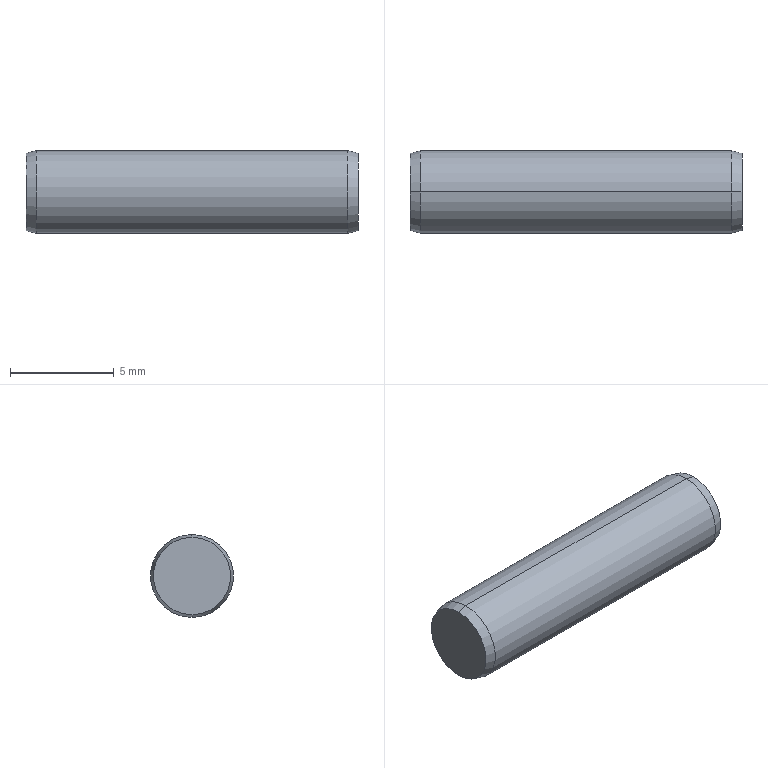Part | STEP file | GB/T 119 4×16 | 1 solid | 8 faces | box 16 x 4 x 4 mm | volume 200.239 mm3 | cone 4 | cylinder 2 | plane 2 | commonest cylinder face diameters 4 x2
STEP:
#1=CARTESIAN_POINT('',(14.,0.,2.));
#2=VERTEX_POINT('',#1);
#3=CARTESIAN_POINT('',(14.,0.,-2.));
#4=VERTEX_POINT('',#3);
#5=CARTESIAN_POINT('',(14.,0.,0.));
#6=DIRECTION('',(-1.,0.,0.));
#7=DIRECTION('',(0.,0.,1.));
#8=AXIS2_PLACEMENT_3D('',#5,#6,#7);
#9=CIRCLE('',#8,2.);
#10=EDGE_CURVE('',#2,#4,#9,.T.);
#11=ORIENTED_EDGE('',*,*,#10,.T.);
#12=CARTESIAN_POINT('',(-1.,0.,-2.));
#13=VERTEX_POINT('',#12);
#14=CARTESIAN_POINT('',(0.,0.,-2.));
#15=DIRECTION('',(-1.,0.,0.));
#16=VECTOR('',#15,1000.);
#17=LINE('',#14,#16);
#18=EDGE_CURVE('',#4,#13,#17,.T.);
#19=ORIENTED_EDGE('',*,*,#18,.T.);
#20=CARTESIAN_POINT('',(-1.,0.,2.));
#21=VERTEX_POINT('',#20);
#22=CARTESIAN_POINT('',(-1.,0.,0.));
#23=DIRECTION('',(-1.,0.,0.));
#24=DIRECTION('',(0.,0.,1.));
#25=AXIS2_PLACEMENT_3D('',#22,#23,#24);
#26=CIRCLE('',#25,2.);
#27=EDGE_CURVE('',#21,#13,#26,.T.);
#28=ORIENTED_EDGE('',*,*,#27,.F.);
#29=CARTESIAN_POINT('',(0.,0.,2.));
#30=DIRECTION('',(-1.,0.,0.));
#31=VECTOR('',#30,1000.);
#32=LINE('',#29,#31);
#33=EDGE_CURVE('',#2,#21,#32,.T.);
#34=ORIENTED_EDGE('',*,*,#33,.F.);
#35=EDGE_LOOP('',(#11,#19,#28,#34));
#36=FACE_OUTER_BOUND('',#35,.T.);
#37=CARTESIAN_POINT('',(0.,0.,0.));
#38=DIRECTION('',(-1.,0.,0.));
#39=DIRECTION('',(0.,0.,1.));
#40=AXIS2_PLACEMENT_3D('',#37,#38,#39);
#41=CYLINDRICAL_SURFACE('',#40,2.);
#42=ADVANCED_FACE('',(#36),#41,.T.);
#43=CARTESIAN_POINT('',(-1.5,0.,1.866));
#44=VERTEX_POINT('',#43);
#45=CARTESIAN_POINT('',(-1.5,0.,-1.866));
#46=VERTEX_POINT('',#45);
#47=CARTESIAN_POINT('',(-1.5,0.,0.));
#48=DIRECTION('',(-1.,0.,0.));
#49=DIRECTION('',(0.,0.,1.));
#50=AXIS2_PLACEMENT_3D('',#47,#48,#49);
#51=CIRCLE('',#50,1.866);
#52=EDGE_CURVE('',#44,#46,#51,.T.);
#53=ORIENTED_EDGE('',*,*,#52,.F.);
#54=CARTESIAN_POINT('',(-1.,0.,2.));
#55=DIRECTION('',(0.9659,0.,0.2588));
#56=VECTOR('',#55,1000.);
#57=LINE('',#54,#56);
#58=EDGE_CURVE('',#44,#21,#57,.T.);
#59=ORIENTED_EDGE('',*,*,#58,.T.);
#60=ORIENTED_EDGE('',*,*,#27,.T.);
#61=CARTESIAN_POINT('',(-1.,0.,-2.));
#62=DIRECTION('',(0.9659,0.,-0.2588));
#63=VECTOR('',#62,1000.);
#64=LINE('',#61,#63);
#65=EDGE_CURVE('',#46,#13,#64,.T.);
#66=ORIENTED_EDGE('',*,*,#65,.F.);
#67=EDGE_LOOP('',(#53,#59,#60,#66));
#68=FACE_OUTER_BOUND('',#67,.T.);
#69=CARTESIAN_POINT('',(-1.,0.,0.));
#70=DIRECTION('',(1.,0.,0.));
#71=DIRECTION('',(0.,0.,-1.));
#72=AXIS2_PLACEMENT_3D('',#69,#70,#71);
#73=CONICAL_SURFACE('',#72,2.,0.2618);
#74=ADVANCED_FACE('',(#68),#73,.T.);
#75=CARTESIAN_POINT('',(14.5,0.,1.866));
#76=VERTEX_POINT('',#75);
#77=CARTESIAN_POINT('',(14.5,0.,-1.866));
#78=VERTEX_POINT('',#77);
#79=CARTESIAN_POINT('',(14.5,0.,0.));
#80=DIRECTION('',(-1.,0.,0.));
#81=DIRECTION('',(0.,0.,1.));
#82=AXIS2_PLACEMENT_3D('',#79,#80,#81);
#83=CIRCLE('',#82,1.866);
#84=EDGE_CURVE('',#76,#78,#83,.T.);
#85=ORIENTED_EDGE('',*,*,#84,.T.);
#86=CARTESIAN_POINT('',(14.5,0.,-1.866));
#87=DIRECTION('',(-0.9659,0.,-0.2588));
#88=VECTOR('',#87,1000.);
#89=LINE('',#86,#88);
#90=EDGE_CURVE('',#78,#4,#89,.T.);
#91=ORIENTED_EDGE('',*,*,#90,.T.);
#92=ORIENTED_EDGE('',*,*,#10,.F.);
#93=CARTESIAN_POINT('',(14.5,0.,1.866));
#94=DIRECTION('',(-0.9659,0.,0.2588));
#95=VECTOR('',#94,1000.);
#96=LINE('',#93,#95);
#97=EDGE_CURVE('',#76,#2,#96,.T.);
#98=ORIENTED_EDGE('',*,*,#97,.F.);
#99=EDGE_LOOP('',(#85,#91,#92,#98));
#100=FACE_OUTER_BOUND('',#99,.T.);
#101=CARTESIAN_POINT('',(14.5,0.,0.));
#102=DIRECTION('',(-1.,0.,0.));
#103=DIRECTION('',(0.,0.,1.));
#104=AXIS2_PLACEMENT_3D('',#101,#102,#103);
#105=CONICAL_SURFACE('',#104,1.866,0.2618);
#106=ADVANCED_FACE('',(#100),#105,.T.);
#107=ORIENTED_EDGE('',*,*,#90,.F.);
#108=CARTESIAN_POINT('',(14.5,0.,0.));
#109=DIRECTION('',(-1.,0.,0.));
#110=DIRECTION('',(0.,0.,1.));
#111=AXIS2_PLACEMENT_3D('',#108,#109,#110);
#112=CIRCLE('',#111,1.866);
#113=EDGE_CURVE('',#78,#76,#112,.T.);
#114=ORIENTED_EDGE('',*,*,#113,.T.);
#115=ORIENTED_EDGE('',*,*,#97,.T.);
#116=CARTESIAN_POINT('',(14.,0.,0.));
#117=DIRECTION('',(-1.,0.,0.));
#118=DIRECTION('',(0.,0.,1.));
#119=AXIS2_PLACEMENT_3D('',#116,#117,#118);
#120=CIRCLE('',#119,2.);
#121=EDGE_CURVE('',#4,#2,#120,.T.);
#122=ORIENTED_EDGE('',*,*,#121,.F.);
#123=EDGE_LOOP('',(#107,#114,#115,#122));
#124=FACE_OUTER_BOUND('',#123,.T.);
#125=CARTESIAN_POINT('',(14.5,0.,0.));
#126=DIRECTION('',(-1.,0.,0.));
#127=DIRECTION('',(0.,0.,1.));
#128=AXIS2_PLACEMENT_3D('',#125,#126,#127);
#129=CONICAL_SURFACE('',#128,1.866,0.2618);
#130=ADVANCED_FACE('',(#124),#129,.T.);
#131=ORIENTED_EDGE('',*,*,#84,.F.);
#132=ORIENTED_EDGE('',*,*,#113,.F.);
#133=EDGE_LOOP('',(#131,#132));
#134=FACE_OUTER_BOUND('',#133,.T.);
#135=CARTESIAN_POINT('',(14.5,1.866,0.));
#136=DIRECTION('',(-1.,0.,0.));
#137=DIRECTION('',(0.,0.,1.));
#138=AXIS2_PLACEMENT_3D('',#135,#136,#137);
#139=PLANE('',#138);
#140=ADVANCED_FACE('',(#134),#139,.F.);
#141=CARTESIAN_POINT('',(-1.5,0.,0.));
#142=DIRECTION('',(-1.,0.,0.));
#143=DIRECTION('',(0.,0.,1.));
#144=AXIS2_PLACEMENT_3D('',#141,#142,#143);
#145=CIRCLE('',#144,1.866);
#146=EDGE_CURVE('',#46,#44,#145,.T.);
#147=ORIENTED_EDGE('',*,*,#146,.T.);
#148=ORIENTED_EDGE('',*,*,#52,.T.);
#149=EDGE_LOOP('',(#147,#148));
#150=FACE_OUTER_BOUND('',#149,.T.);
#151=CARTESIAN_POINT('',(-1.5,1.866,0.));
#152=DIRECTION('',(1.,0.,0.));
#153=DIRECTION('',(0.,0.,-1.));
#154=AXIS2_PLACEMENT_3D('',#151,#152,#153);
#155=PLANE('',#154);
#156=ADVANCED_FACE('',(#150),#155,.F.);
#157=ORIENTED_EDGE('',*,*,#58,.F.);
#158=ORIENTED_EDGE('',*,*,#146,.F.);
#159=ORIENTED_EDGE('',*,*,#65,.T.);
#160=CARTESIAN_POINT('',(-1.,0.,0.));
#161=DIRECTION('',(-1.,0.,0.));
#162=DIRECTION('',(0.,0.,1.));
#163=AXIS2_PLACEMENT_3D('',#160,#161,#162);
#164=CIRCLE('',#163,2.);
#165=EDGE_CURVE('',#13,#21,#164,.T.);
#166=ORIENTED_EDGE('',*,*,#165,.T.);
#167=EDGE_LOOP('',(#157,#158,#159,#166));
#168=FACE_OUTER_BOUND('',#167,.T.);
#169=CARTESIAN_POINT('',(-1.,0.,0.));
#170=DIRECTION('',(1.,0.,0.));
#171=DIRECTION('',(0.,0.,-1.));
#172=AXIS2_PLACEMENT_3D('',#169,#170,#171);
#173=CONICAL_SURFACE('',#172,2.,0.2618);
#174=ADVANCED_FACE('',(#168),#173,.T.);
#175=ORIENTED_EDGE('',*,*,#18,.F.);
#176=ORIENTED_EDGE('',*,*,#121,.T.);
#177=ORIENTED_EDGE('',*,*,#33,.T.);
#178=ORIENTED_EDGE('',*,*,#165,.F.);
#179=EDGE_LOOP('',(#175,#176,#177,#178));
#180=FACE_OUTER_BOUND('',#179,.T.);
#181=CARTESIAN_POINT('',(0.,0.,0.));
#182=DIRECTION('',(-1.,0.,0.));
#183=DIRECTION('',(0.,0.,1.));
#184=AXIS2_PLACEMENT_3D('',#181,#182,#183);
#185=CYLINDRICAL_SURFACE('',#184,2.);
#186=ADVANCED_FACE('',(#180),#185,.T.);
#187=CLOSED_SHELL('',(#42,#74,#106,#130,#140,#156,#174,#186));
#188=MANIFOLD_SOLID_BREP('',#187);
#189=CARTESIAN_POINT('',(0.,0.,0.));
#190=DIRECTION('',(0.,0.,1.));
#191=DIRECTION('',(1.,0.,0.));
#192=AXIS2_PLACEMENT_3D('',#189,#190,#191);
#193=(LENGTH_UNIT()NAMED_UNIT(*)SI_UNIT(.MILLI.,.METRE.));
#194=UNCERTAINTY_MEASURE_WITH_UNIT(LENGTH_MEASURE(0.00001),#193,'','');
#195=(NAMED_UNIT(*)PLANE_ANGLE_UNIT()SI_UNIT($,.RADIAN.));
#196=(NAMED_UNIT(*)SI_UNIT($,.STERADIAN.)SOLID_ANGLE_UNIT());
#197=(GEOMETRIC_REPRESENTATION_CONTEXT(3)GLOBAL_UNCERTAINTY_ASSIGNED_CONTEXT((#194))GLOBAL_UNIT_ASSIGNED_CONTEXT((#193,#195,#196))REPRESENTATION_CONTEXT('',''));
#198=ADVANCED_BREP_SHAPE_REPRESENTATION('',(#188,#192),#197);